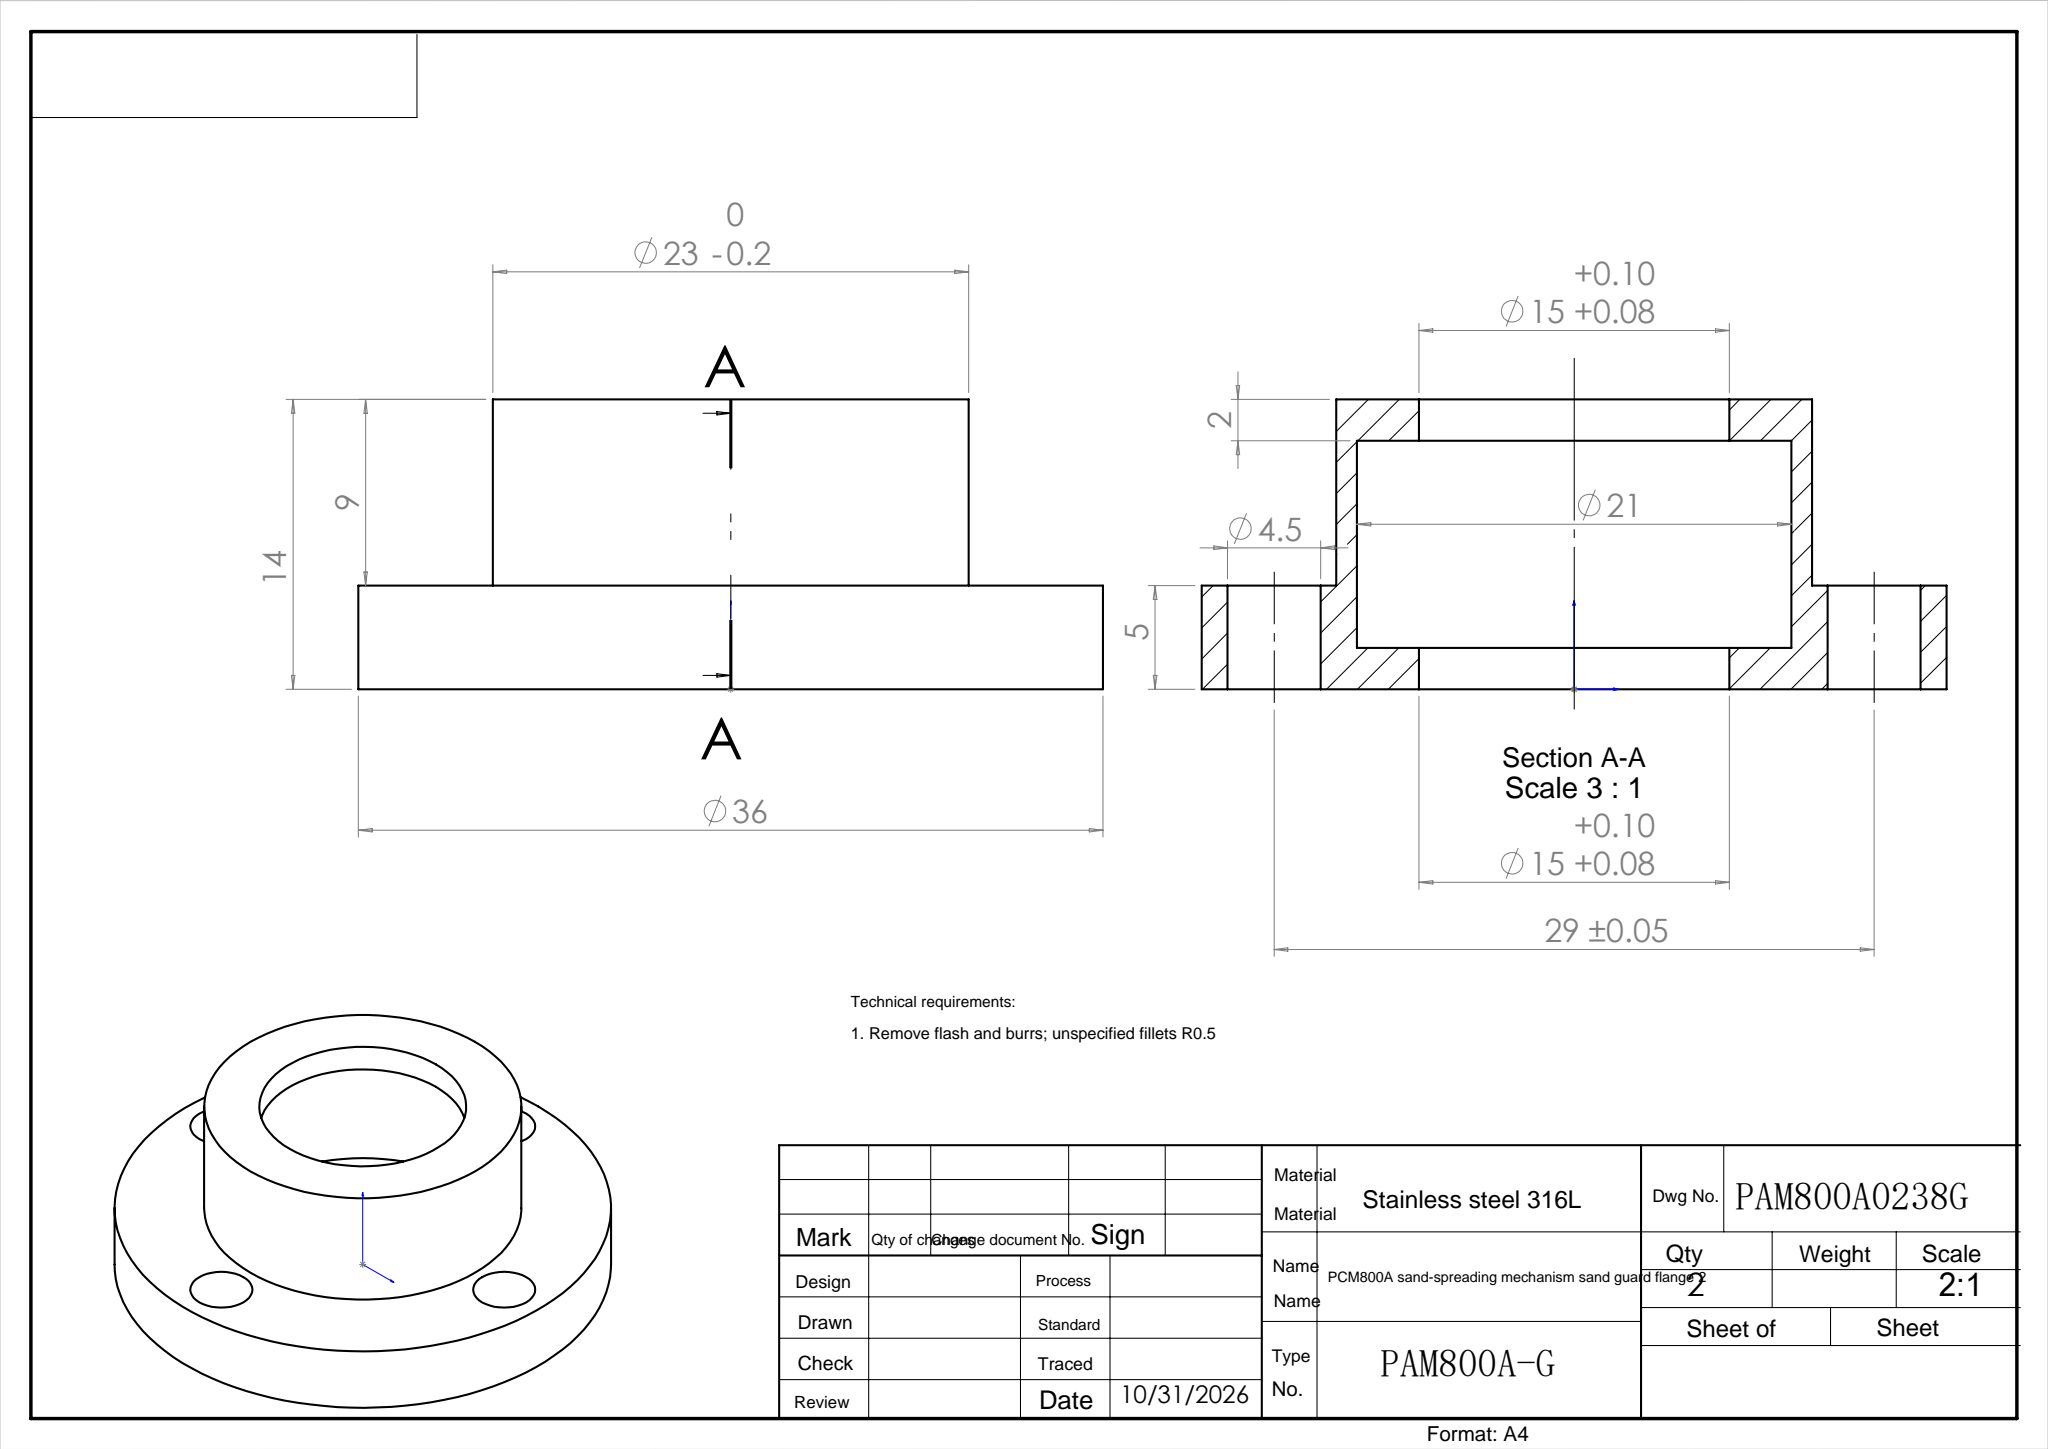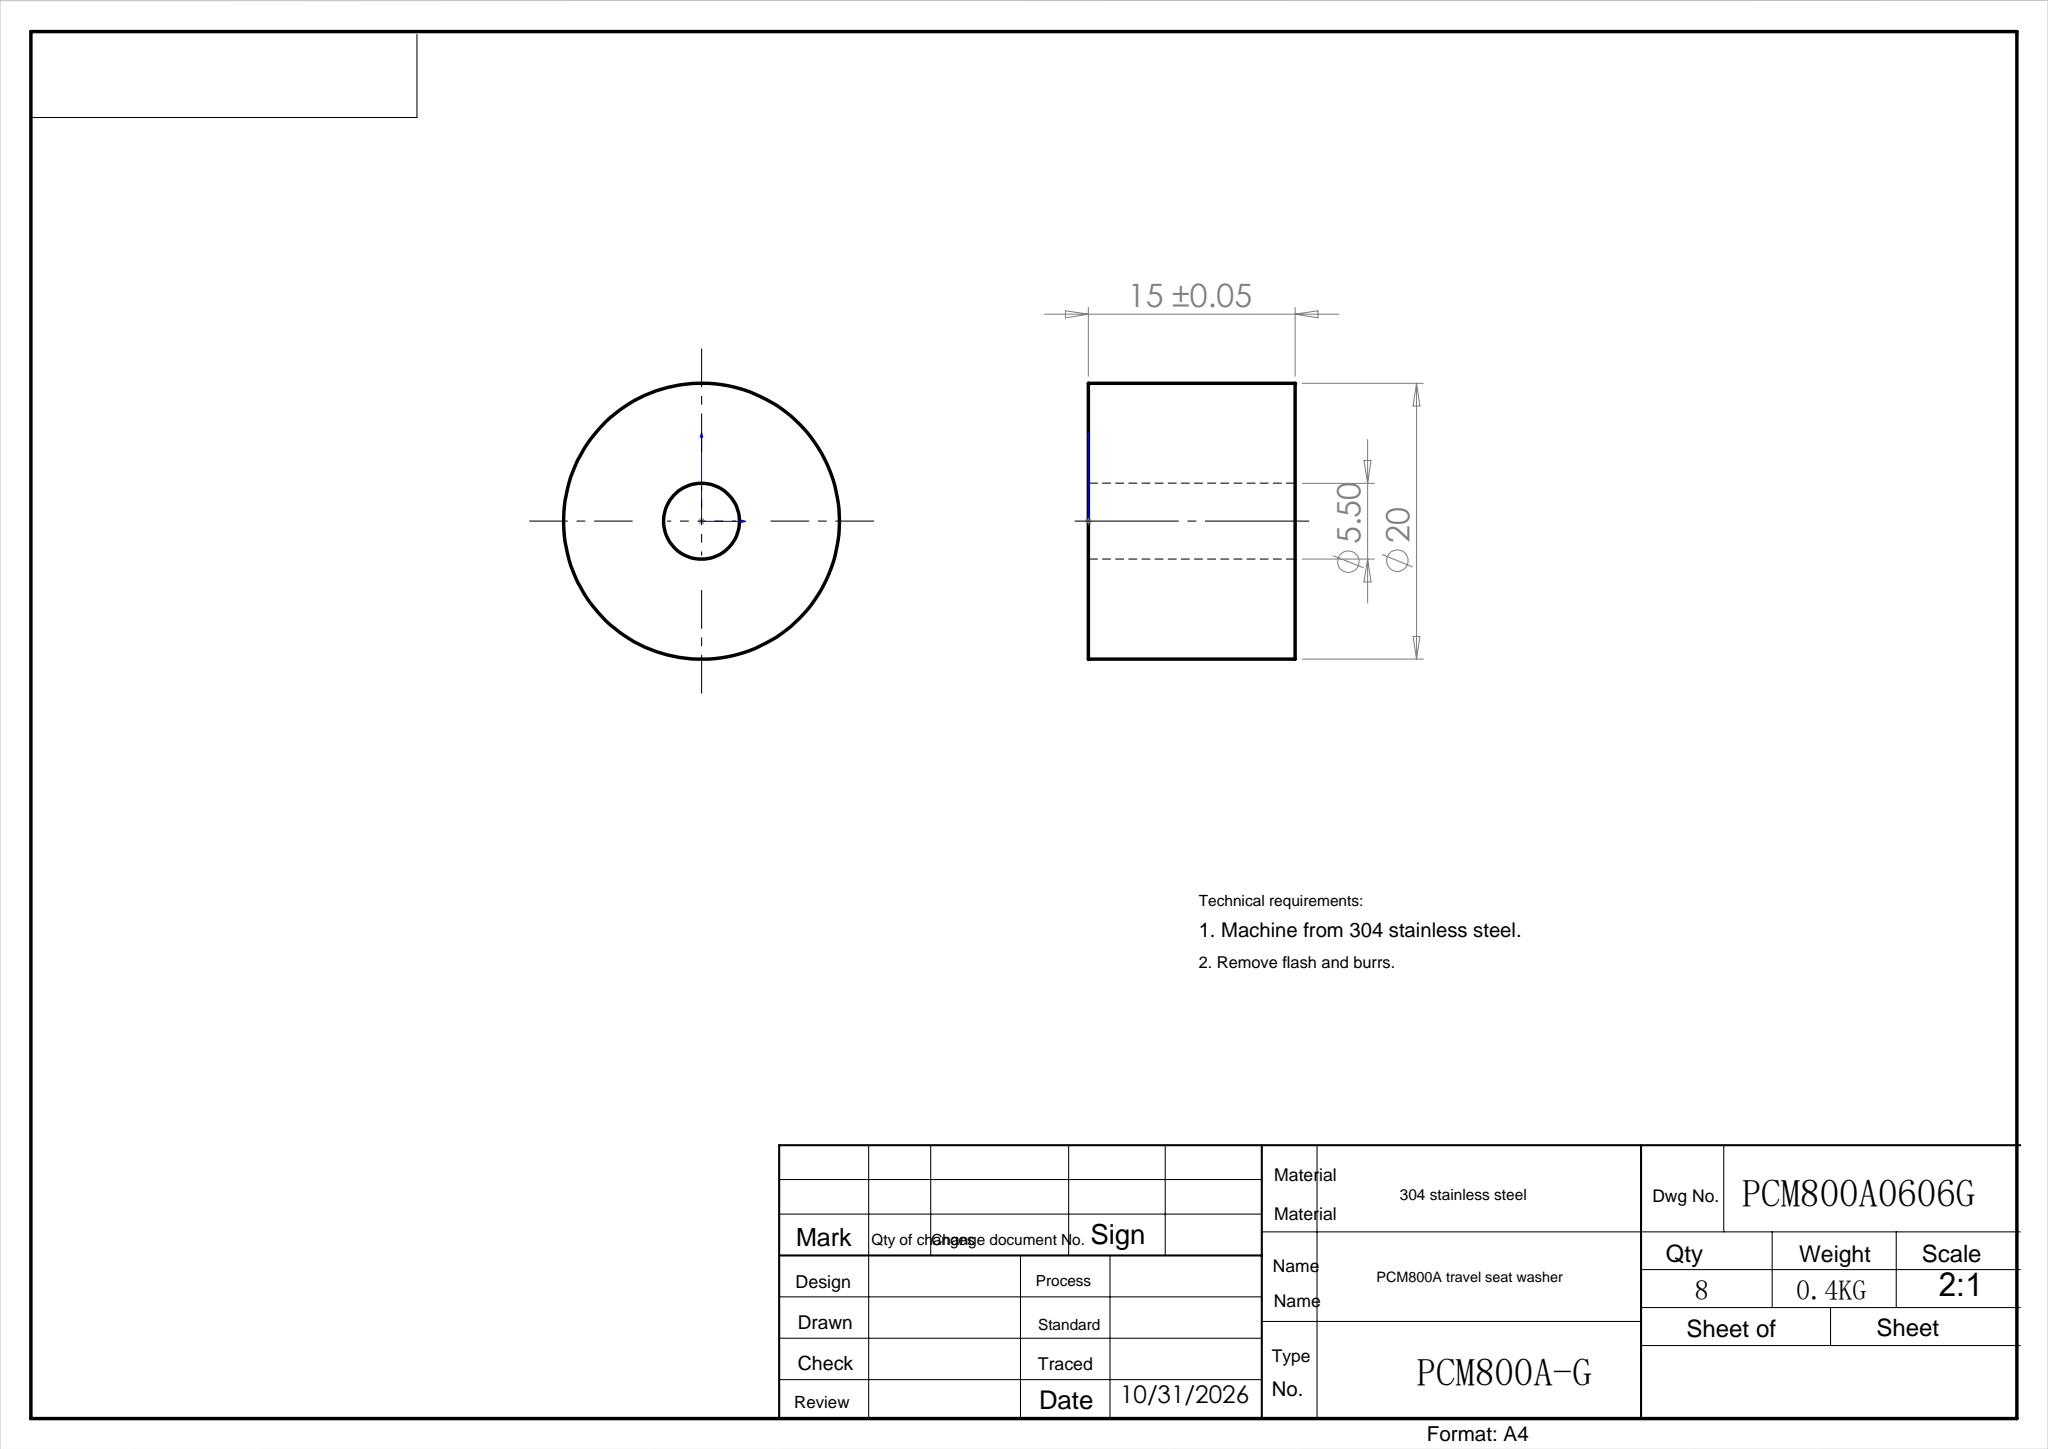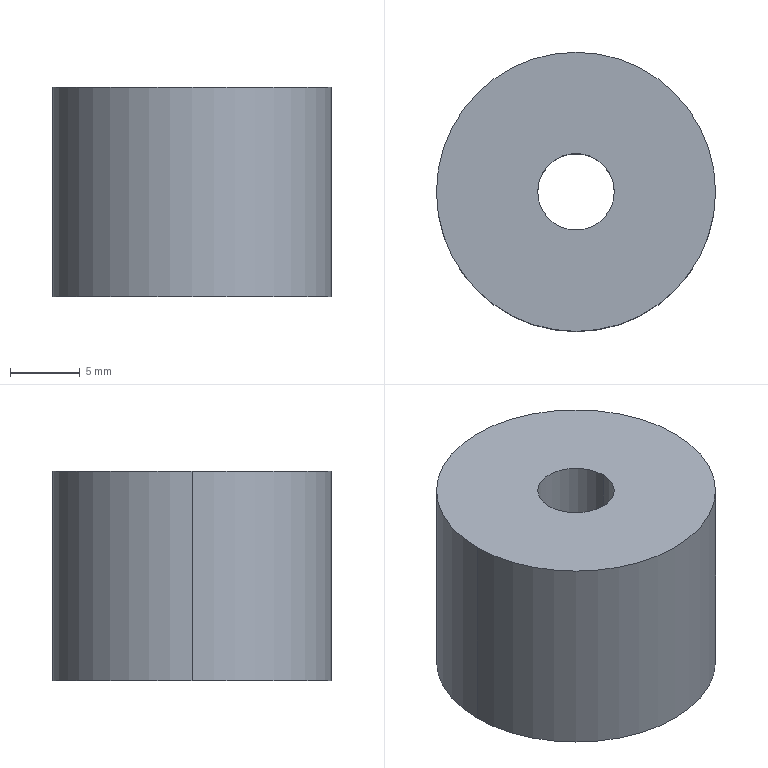Part | SolidWorks | features Extrusion 1 | 1 solid | 6 faces | box 20 x 20 x 15 mm | volume 4356 mm3 | cylinder 4 | plane 2 | commonest cylinder face diameters 5.5 x2 20 x2
STEP:
#1=CARTESIAN_POINT('',(-2.75,0.,15.));
#2=VERTEX_POINT('',#1);
#3=CARTESIAN_POINT('',(2.75,0.,15.));
#4=VERTEX_POINT('',#3);
#5=CARTESIAN_POINT('',(0.,0.,15.));
#6=DIRECTION('',(0.,0.,1.));
#7=DIRECTION('',(1.,0.,0.));
#8=AXIS2_PLACEMENT_3D('',#5,#6,#7);
#9=CIRCLE('',#8,2.75);
#10=EDGE_CURVE('',#2,#4,#9,.T.);
#11=ORIENTED_EDGE('',*,*,#10,.T.);
#12=CARTESIAN_POINT('',(2.75,0.,0.));
#13=VERTEX_POINT('',#12);
#14=CARTESIAN_POINT('',(2.75,0.,15.));
#15=DIRECTION('',(0.,0.,-1.));
#16=VECTOR('',#15,1000.);
#17=LINE('',#14,#16);
#18=EDGE_CURVE('',#4,#13,#17,.T.);
#19=ORIENTED_EDGE('',*,*,#18,.T.);
#20=CARTESIAN_POINT('',(-2.75,0.,0.));
#21=VERTEX_POINT('',#20);
#22=CARTESIAN_POINT('',(0.,0.,0.));
#23=DIRECTION('',(0.,0.,1.));
#24=DIRECTION('',(1.,0.,0.));
#25=AXIS2_PLACEMENT_3D('',#22,#23,#24);
#26=CIRCLE('',#25,2.75);
#27=EDGE_CURVE('',#21,#13,#26,.T.);
#28=ORIENTED_EDGE('',*,*,#27,.F.);
#29=CARTESIAN_POINT('',(-2.75,0.,15.));
#30=DIRECTION('',(0.,0.,-1.));
#31=VECTOR('',#30,1000.);
#32=LINE('',#29,#31);
#33=EDGE_CURVE('',#2,#21,#32,.T.);
#34=ORIENTED_EDGE('',*,*,#33,.F.);
#35=EDGE_LOOP('',(#11,#19,#28,#34));
#36=FACE_OUTER_BOUND('',#35,.T.);
#37=CARTESIAN_POINT('',(0.,0.,15.));
#38=DIRECTION('',(0.,0.,-1.));
#39=DIRECTION('',(-1.,0.,0.));
#40=AXIS2_PLACEMENT_3D('',#37,#38,#39);
#41=CYLINDRICAL_SURFACE('',#40,2.75);
#42=ADVANCED_FACE('',(#36),#41,.F.);
#43=CARTESIAN_POINT('',(10.,0.,15.));
#44=VERTEX_POINT('',#43);
#45=CARTESIAN_POINT('',(-10.,0.,15.));
#46=VERTEX_POINT('',#45);
#47=CARTESIAN_POINT('',(0.,0.,15.));
#48=DIRECTION('',(0.,0.,1.));
#49=DIRECTION('',(1.,0.,0.));
#50=AXIS2_PLACEMENT_3D('',#47,#48,#49);
#51=CIRCLE('',#50,10.);
#52=EDGE_CURVE('',#44,#46,#51,.T.);
#53=ORIENTED_EDGE('',*,*,#52,.F.);
#54=CARTESIAN_POINT('',(10.,0.,0.));
#55=VERTEX_POINT('',#54);
#56=CARTESIAN_POINT('',(10.,0.,15.));
#57=DIRECTION('',(0.,0.,-1.));
#58=VECTOR('',#57,1000.);
#59=LINE('',#56,#58);
#60=EDGE_CURVE('',#44,#55,#59,.T.);
#61=ORIENTED_EDGE('',*,*,#60,.T.);
#62=CARTESIAN_POINT('',(-10.,0.,0.));
#63=VERTEX_POINT('',#62);
#64=CARTESIAN_POINT('',(0.,0.,0.));
#65=DIRECTION('',(0.,0.,1.));
#66=DIRECTION('',(1.,0.,0.));
#67=AXIS2_PLACEMENT_3D('',#64,#65,#66);
#68=CIRCLE('',#67,10.);
#69=EDGE_CURVE('',#55,#63,#68,.T.);
#70=ORIENTED_EDGE('',*,*,#69,.T.);
#71=CARTESIAN_POINT('',(-10.,0.,15.));
#72=DIRECTION('',(0.,0.,-1.));
#73=VECTOR('',#72,1000.);
#74=LINE('',#71,#73);
#75=EDGE_CURVE('',#46,#63,#74,.T.);
#76=ORIENTED_EDGE('',*,*,#75,.F.);
#77=EDGE_LOOP('',(#53,#61,#70,#76));
#78=FACE_OUTER_BOUND('',#77,.T.);
#79=CARTESIAN_POINT('',(0.,0.,15.));
#80=DIRECTION('',(0.,0.,-1.));
#81=DIRECTION('',(-1.,0.,0.));
#82=AXIS2_PLACEMENT_3D('',#79,#80,#81);
#83=CYLINDRICAL_SURFACE('',#82,10.);
#84=ADVANCED_FACE('',(#78),#83,.T.);
#85=CARTESIAN_POINT('',(0.,0.,15.));
#86=DIRECTION('',(0.,0.,1.));
#87=DIRECTION('',(1.,0.,0.));
#88=AXIS2_PLACEMENT_3D('',#85,#86,#87);
#89=CIRCLE('',#88,10.);
#90=EDGE_CURVE('',#46,#44,#89,.T.);
#91=ORIENTED_EDGE('',*,*,#90,.T.);
#92=ORIENTED_EDGE('',*,*,#52,.T.);
#93=EDGE_LOOP('',(#91,#92));
#94=FACE_OUTER_BOUND('',#93,.T.);
#95=ORIENTED_EDGE('',*,*,#10,.F.);
#96=CARTESIAN_POINT('',(0.,0.,15.));
#97=DIRECTION('',(0.,0.,1.));
#98=DIRECTION('',(1.,0.,0.));
#99=AXIS2_PLACEMENT_3D('',#96,#97,#98);
#100=CIRCLE('',#99,2.75);
#101=EDGE_CURVE('',#4,#2,#100,.T.);
#102=ORIENTED_EDGE('',*,*,#101,.F.);
#103=EDGE_LOOP('',(#95,#102));
#104=FACE_BOUND('',#103,.T.);
#105=CARTESIAN_POINT('',(0.,0.,15.));
#106=DIRECTION('',(0.,0.,1.));
#107=DIRECTION('',(1.,0.,0.));
#108=AXIS2_PLACEMENT_3D('',#105,#106,#107);
#109=PLANE('',#108);
#110=ADVANCED_FACE('',(#94,#104),#109,.T.);
#111=CARTESIAN_POINT('',(0.,0.,0.));
#112=DIRECTION('',(0.,0.,1.));
#113=DIRECTION('',(1.,0.,0.));
#114=AXIS2_PLACEMENT_3D('',#111,#112,#113);
#115=CIRCLE('',#114,10.);
#116=EDGE_CURVE('',#63,#55,#115,.T.);
#117=ORIENTED_EDGE('',*,*,#116,.F.);
#118=ORIENTED_EDGE('',*,*,#69,.F.);
#119=EDGE_LOOP('',(#117,#118));
#120=FACE_OUTER_BOUND('',#119,.T.);
#121=ORIENTED_EDGE('',*,*,#27,.T.);
#122=CARTESIAN_POINT('',(0.,0.,0.));
#123=DIRECTION('',(0.,0.,1.));
#124=DIRECTION('',(1.,0.,0.));
#125=AXIS2_PLACEMENT_3D('',#122,#123,#124);
#126=CIRCLE('',#125,2.75);
#127=EDGE_CURVE('',#13,#21,#126,.T.);
#128=ORIENTED_EDGE('',*,*,#127,.T.);
#129=EDGE_LOOP('',(#121,#128));
#130=FACE_BOUND('',#129,.T.);
#131=CARTESIAN_POINT('',(0.,0.,0.));
#132=DIRECTION('',(0.,0.,1.));
#133=DIRECTION('',(1.,0.,0.));
#134=AXIS2_PLACEMENT_3D('',#131,#132,#133);
#135=PLANE('',#134);
#136=ADVANCED_FACE('',(#120,#130),#135,.F.);
#137=ORIENTED_EDGE('',*,*,#60,.F.);
#138=ORIENTED_EDGE('',*,*,#90,.F.);
#139=ORIENTED_EDGE('',*,*,#75,.T.);
#140=ORIENTED_EDGE('',*,*,#116,.T.);
#141=EDGE_LOOP('',(#137,#138,#139,#140));
#142=FACE_OUTER_BOUND('',#141,.T.);
#143=CARTESIAN_POINT('',(0.,0.,15.));
#144=DIRECTION('',(0.,0.,-1.));
#145=DIRECTION('',(-1.,0.,0.));
#146=AXIS2_PLACEMENT_3D('',#143,#144,#145);
#147=CYLINDRICAL_SURFACE('',#146,10.);
#148=ADVANCED_FACE('',(#142),#147,.T.);
#149=ORIENTED_EDGE('',*,*,#18,.F.);
#150=ORIENTED_EDGE('',*,*,#101,.T.);
#151=ORIENTED_EDGE('',*,*,#33,.T.);
#152=ORIENTED_EDGE('',*,*,#127,.F.);
#153=EDGE_LOOP('',(#149,#150,#151,#152));
#154=FACE_OUTER_BOUND('',#153,.T.);
#155=CARTESIAN_POINT('',(0.,0.,15.));
#156=DIRECTION('',(0.,0.,-1.));
#157=DIRECTION('',(-1.,0.,0.));
#158=AXIS2_PLACEMENT_3D('',#155,#156,#157);
#159=CYLINDRICAL_SURFACE('',#158,2.75);
#160=ADVANCED_FACE('',(#154),#159,.F.);
#161=CLOSED_SHELL('',(#42,#84,#110,#136,#148,#160));
#162=MANIFOLD_SOLID_BREP('',#161);
#163=CARTESIAN_POINT('',(0.,0.,0.));
#164=DIRECTION('',(0.,0.,1.));
#165=DIRECTION('',(1.,0.,0.));
#166=AXIS2_PLACEMENT_3D('',#163,#164,#165);
#167=(LENGTH_UNIT()NAMED_UNIT(*)SI_UNIT(.MILLI.,.METRE.));
#168=UNCERTAINTY_MEASURE_WITH_UNIT(LENGTH_MEASURE(0.00001),#167,'','');
#169=(NAMED_UNIT(*)PLANE_ANGLE_UNIT()SI_UNIT($,.RADIAN.));
#170=(NAMED_UNIT(*)SI_UNIT($,.STERADIAN.)SOLID_ANGLE_UNIT());
#171=(GEOMETRIC_REPRESENTATION_CONTEXT(3)GLOBAL_UNCERTAINTY_ASSIGNED_CONTEXT((#168))GLOBAL_UNIT_ASSIGNED_CONTEXT((#167,#169,#170))REPRESENTATION_CONTEXT('',''));
#172=ADVANCED_BREP_SHAPE_REPRESENTATION('',(#162,#166),#171);